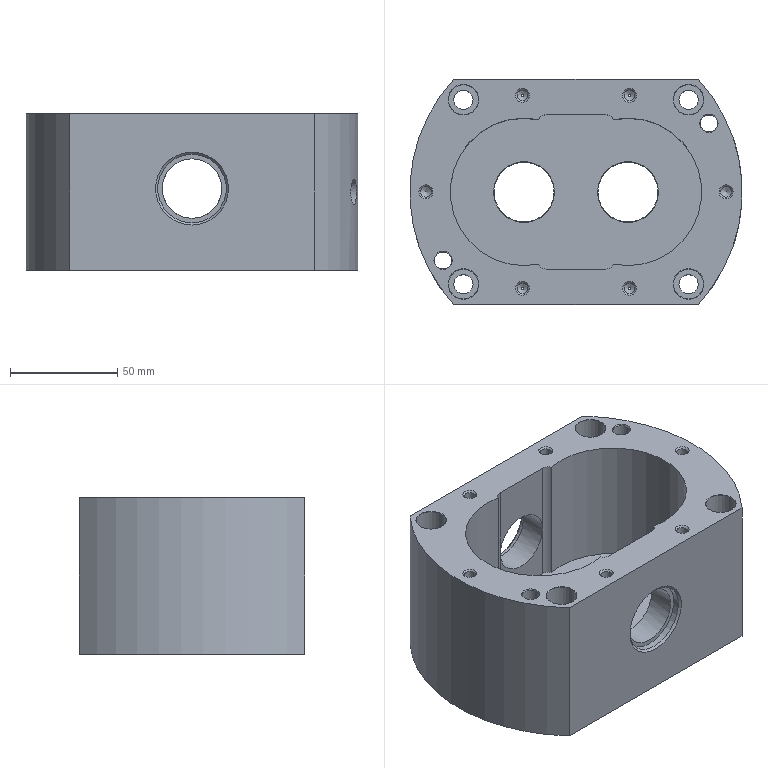NC program | NX | posted with a generic post | part box 155 x 105 x 73.2 mm
Lines 21970 to 22392 of 150882:
(FLOOR_WALL_2 , TOOL : D6JING)
N43890 T16 M6
N43892 G54
N43894 G17 G0 G90 X40.24 Y-44.486 B0. C0. S5000 M3
N43896 G43 Z30. H16
N43898 Z-1.
N43900 G94 G1 Z-2. F1000.
N43902 G3 X40.7 Y-44.7 R0.6
N43904 G1 X-40.7
N43906 Y-40.105
N43908 G3 X-40.188 Y-38.45 R6.3
N43910 G1 X-39.834 Y-36.282
N43912 G3 X-39.995 Y-35.966 R0.3
N43914 G1 X-41.955 Y-34.974
N43916 G2 X-49.587 Y-29.911 R39.2
N43918 G1 X-51.263 Y-28.491
N43920 G3 X-51.617 Y-28.466 R0.3
N43922 G1 X-53.477 Y-29.635
N43924 G3 X-54.757 Y-30.7 R6.3
N43926 G1 X-62.575
N43928 G2 X-66.236 Y21.7 R69.7
N43930 G1 X-61.75
N43932 G3 X-60.197 Y20.982 R6.3
N43934 G1 X-58.097 Y20.338
N43936 G3 X-57.762 Y20.455 R0.3
N43938 G1 X-56.515 Y22.263
N43940 G2 X-41.955 Y34.974 R39.2
N43942 G1 X-39.995 Y35.966
N43944 G3 X-39.834 Y36.282 R0.3
N43946 G1 X-40.188 Y38.45
N43948 G3 X-40.7 Y40.105 R6.3
N43950 G1 Y44.7
N43952 X40.7
N43954 Y40.105
N43956 G3 X40.188 Y38.45 R6.3
N43958 G1 X39.834 Y36.282
N43960 G3 X39.995 Y35.966 R0.3
N43962 G1 X41.955 Y34.974
N43964 G2 X49.587 Y29.911 R39.2
N43966 G1 X51.263 Y28.491
N43968 G3 X51.617 Y28.466 R0.3
N43970 G1 X53.477 Y29.635
N43972 G3 X54.757 Y30.7 R6.3
N43974 G1 X62.575
N43976 G2 X66.236 Y-21.7 R69.7
N43978 G1 X61.75
N43980 G3 X60.197 Y-20.982 R6.3
N43982 G1 X58.097 Y-20.338
N43984 G3 X57.762 Y-20.455 R0.3
N43986 G1 X56.515 Y-22.263
N43988 G2 X41.955 Y-34.974 R39.2
N43990 G1 X39.995 Y-35.966
N43992 G3 X39.834 Y-36.282 R0.3
N43994 G1 X40.188 Y-38.45
N43996 G3 X40.7 Y-40.105 R6.3
N43998 G1 Y-44.7
N44000 X37.7 Y-41.7
N44002 X-37.7
N44004 Y-40.705
N44006 G3 X-37.228 Y-38.934 R9.3
N44008 G1 X-36.874 Y-36.766
N44010 G3 X-38.64 Y-33.29 R3.3
N44012 G1 X-40.6 Y-32.297
N44014 G2 X-47.648 Y-27.622 R36.2
N44016 G1 X-49.324 Y-26.202
N44018 G3 X-53.214 Y-25.926 R3.3
N44020 G1 X-55.073 Y-27.095
N44022 G3 X-55.925 Y-27.7 R9.3
N44024 G1 X-60.676
N44026 G2 X-64.025 Y18.7 R66.7
N44028 G1 X-62.537
N44030 G3 X-61.076 Y18.113 R9.3
N44032 G1 X-58.976 Y17.47
N44034 G3 X-57.242 Y17.415 R3.3
N44036 G1 X-56.545 Y14.498
N44038 G3 X-51.643 Y-22.423 R35.4
N44040 X-54.876 Y-23.427 R6.3
N44042 G1 X-56.67 Y-24.555
N44044 G3 X-56.895 Y-24.7 R12.3
N44046 G1 X-58.716
N44048 G2 X-60.542 Y-19.808 R63.7
N44050 G1 X-57.691 Y-18.876
N44052 G3 X-56.472 Y-20.887 R38.4
N44054 G1 X-56.895 Y-21.153
N44056 G2 X-57.691 Y-18.876 R60.7
N44058 G1 X-60.542 Y-19.808
N44060 G2 X-61.856 Y15.215 R63.7
N44062 G1 X-59.854 Y14.601
N44064 G3 X-56.545 Y14.498 R6.3
N44066 G1 X-57.242 Y17.415
N44068 G3 X-55.293 Y18.751 R3.3
N44070 G1 X-54.045 Y20.559
N44072 G2 X-40.6 Y32.297 R36.2
N44074 G1 X-38.64 Y33.29
N44076 G3 X-36.874 Y36.766 R3.3
N44078 G1 X-37.228 Y38.934
N44080 G3 X-37.7 Y40.705 R9.3
N44082 G1 Y41.7
N44084 X37.7
N44086 Y40.705
N44088 G3 X37.228 Y38.934 R9.3
N44090 G1 X36.874 Y36.766
N44092 G3 X37.054 Y35.041 R3.3
N44094 G1 X34.257 Y33.956
N44096 G3 X1.238 Y26.9 R35.4
N44098 G1 X-1.238
N44100 G3 X-34.257 Y33.956 R35.4
N44102 X-33.913 Y37.249 R6.3
N44104 G1 X-34.15 Y38.7
N44106 X10.105
N44108 Y35.7
N44110 G3 X0.155 Y29.9 R38.4
N44112 G1 X-0.155
N44114 G3 X-10.105 Y35.7 R38.4
N44116 G1 X10.105
N44118 Y38.7
N44120 X34.15
N44122 X33.913 Y37.249
N44124 G3 X34.257 Y33.956 R6.3
N44126 G1 X37.054 Y35.041
N44128 G3 X38.64 Y33.29 R3.3
N44130 G1 X40.6 Y32.297
N44132 G2 X47.648 Y27.622 R36.2
N44134 G1 X49.324 Y26.202
N44136 G3 X53.214 Y25.926 R3.3
N44138 G1 X55.073 Y27.095
N44140 G3 X55.925 Y27.7 R9.3
N44142 G1 X60.676
N44144 G2 X64.025 Y-18.7 R66.7
N44146 G1 X62.537
N44148 G3 X61.076 Y-18.113 R9.3
N44150 G1 X58.976 Y-17.47
N44152 G3 X57.242 Y-17.415 R3.3
N44154 G1 X56.545 Y-14.498
N44156 G3 X51.643 Y22.423 R35.4
N44158 X54.876 Y23.427 R6.3
N44160 G1 X56.67 Y24.555
N44162 G3 X56.895 Y24.7 R12.3
N44164 G1 X58.716
N44166 G2 X60.542 Y19.809 R63.7
N44168 G1 X57.691 Y18.876
N44170 G3 X56.472 Y20.887 R38.4
N44172 G1 X56.895 Y21.153
N44174 G2 X57.691 Y18.876 R60.7
N44176 G1 X60.542 Y19.809
N44178 G2 X61.856 Y-15.215 R63.7
N44180 G1 X59.854 Y-14.601
N44182 G3 X56.545 Y-14.498 R6.3
N44184 G1 X57.242 Y-17.415
N44186 G3 X55.293 Y-18.751 R3.3
N44188 G1 X54.045 Y-20.559
N44190 G2 X40.6 Y-32.297 R36.2
N44192 G1 X38.64 Y-33.29
N44194 G3 X36.874 Y-36.766 R3.3
N44196 G1 X37.228 Y-38.934
N44198 G3 X37.7 Y-40.705 R9.3
N44200 G1 Y-41.7
N44202 X34.15 Y-38.7
N44204 X-34.15
N44206 X-33.913 Y-37.249
N44208 G3 X-34.257 Y-33.956 R6.3
N44210 X-1.238 Y-26.9 R35.4
N44212 G1 X1.238
N44214 G3 X11.21 Y-32.911 R35.4
N44216 G1 X10.105 Y-35.7
N44218 X-10.105
N44220 G3 X-0.155 Y-29.9 R38.4
N44222 G1 X0.155
N44224 G3 X10.105 Y-35.7 R38.4
N44226 G1 X11.21 Y-32.911
N44228 G3 X34.257 Y-33.956 R35.4
N44230 G1 X34.087 Y-33.381
N44232 G2 X1.461 Y-26.3 R34.8
N44234 G1 X-1.461
N44236 G2 X-1.461 Y26.3 R-34.8
N44238 G1 X1.461
N44240 G2 X34.087 Y-33.381 R-34.8
N44242 G1 X34.257 Y-33.956
N44244 G3 X33.913 Y-37.249 R6.3
N44246 G1 X34.15 Y-38.7
N44248 X33.298 Y-33.517
N44250 G3 X32.8 Y-33.424 R0.6
N44252 G2 X1.573 Y-26. R34.5
N44254 G1 X-1.573
N44256 G2 X-1.573 Y26. R-34.5
N44258 G1 X1.573
N44260 G2 X32.8 Y-33.424 R-34.5
N44262 G3 X32.408 Y-33.745 R0.6
N44264 G1 X31.809 Y-34.993
N44266 Z-1.
N44268 G0 Z30.
N44270 X-1.371 Y-43.7
N44272 Z-1.
N44274 G1 Z-2.
N44276 X-0.46 Y-44.786
N44278 G3 X0. Y-45. R0.6
N44280 G1 X41.
N44282 Y-40.037
N44284 G2 X40.485 Y-38.402 R6.
N44286 G1 X40.13 Y-36.234
N44288 X42.09 Y-35.242
N44290 G3 X56.762 Y-22.433 R39.5
N44292 G1 X58.009 Y-20.625
N44294 X60.109 Y-21.268
N44296 G2 X61.661 Y-22. R6.
N44298 G1 X66.453
N44300 G3 X62.761 Y31. R70.
N44302 G1 X54.624
N44304 G2 X53.317 Y29.889 R6.
N44306 G1 X51.457 Y28.72
N44308 X49.781 Y30.14
N44310 G3 X42.09 Y35.242 R39.5
N44312 G1 X40.13 Y36.234
N44314 X40.485 Y38.402
N44316 G2 X41. Y40.037 R6.
N44318 G1 Y45.
N44320 X-41.
N44322 Y40.037
N44324 G2 X-40.485 Y38.402 R6.
N44326 G1 X-40.13 Y36.234
N44328 X-42.09 Y35.242
N44330 G3 X-56.762 Y22.433 R39.5
N44332 G1 X-58.009 Y20.625
N44334 X-60.109 Y21.268
N44336 G2 X-61.661 Y22. R6.
N44338 G1 X-66.453
N44340 G3 X-62.761 Y-31. R70.
N44342 G1 X-54.624
N44344 G2 X-53.317 Y-29.889 R6.
N44346 G1 X-51.457 Y-28.72
N44348 X-49.781 Y-30.14
N44350 G3 X-42.09 Y-35.242 R39.5
N44352 G1 X-40.13 Y-36.234
N44354 X-40.485 Y-38.402
N44356 G2 X-41. Y-40.037 R6.
N44358 G1 Y-45.
N44360 X0.
N44362 G3 X0.46 Y-44.786 R0.6
N44364 G1 X1.119 Y-44.
N44366 Z-1.
N44368 G0 Z30.
N44370 X-60.222 Y-6.288
N44372 Z-6.
N44374 G1 Z-7.
N44376 G3 X-60.084 Y-5.8 R0.6
N44378 X-0.908 Y-27.8 R36.3
N44380 G1 X0.908
N44382 G3 X0.908 Y27.8 R-36.3
N44384 G1 X-0.908
N44386 G3 X-60.084 Y5.8 R36.3
N44388 G1 X-69.458
N44390 G2 X-66.236 Y21.7 R69.7
N44392 G1 X-61.75
N44394 G3 X-59.002 Y20.739 R6.3
N44396 G1 X-59.311 Y17.755
N44398 G3 X-62.552 Y8.8 R39.3
N44400 G1 X-66.117
N44402 G2 X-64.025 Y18.7 R66.7
N44404 G1 X-62.537
N44406 G3 X-59.311 Y17.755 R9.3
N44408 G1 X-59.002 Y20.739
N44410 G3 X-53.413 Y23.094 R6.3
N44412 G2 X-43.197 Y32.013 R37.2
N44414 G3 X-40.7 Y40.105 R6.3
N44416 G1 Y44.7
N44418 X-5.8
N44420 Y39.
N44422 G3 X-5.5 Y38.7 R0.3
N44424 G1 X5.5
N44426 G3 X5.8 Y39. R0.3
N44428 G1 Y44.7
N44430 X40.7
N44432 Y40.105
N44434 G3 X40.109 Y37.232 R6.3
N44436 G1 X37.111 Y37.136
N44438 G3 X0. Y30.926 R39.3
N44440 X-37.111 Y37.136 R39.3
N44442 X-37.7 Y40.705 R9.3
N44444 G1 Y41.7
N44446 X-8.8
N44448 Y39.
N44450 G3 X-5.5 Y35.7 R3.3
N44452 G1 X5.5
N44454 G3 X8.8 Y39. R3.3
N44456 G1 Y41.7
N44458 X37.7
N44460 Y40.705
N44462 G3 X37.111 Y37.136 R9.3
N44464 G1 X40.109 Y37.232
N44466 G3 X43.197 Y32.013 R6.3
N44468 G2 X46.376 Y29.904 R37.2
N44470 G3 X54.757 Y30.7 R6.3
N44472 G1 X62.575
N44474 G2 X69.458 Y5.8 R69.7
N44476 G1 X62.552
N44478 Y8.8
N44480 G3 X53.463 Y26.289 R39.3
N44482 X55.925 Y27.7 R9.3
N44484 G1 X60.676
N44486 G2 X61.67 Y25.411 R66.7
N44488 G1 X58.896 Y24.268
N44490 G3 X58.589 Y24.7 R42.3
N44492 G1 X58.716
N44494 G2 X58.896 Y24.268 R63.7
N44496 G1 X61.67 Y25.411
N44498 G2 X66.117 Y8.8 R66.7
N44500 G1 X62.552
N44502 Y5.8
N44504 X62.
N44506 G3 X61.7 Y5.5 R0.3
N44508 G1 Y-5.5
N44510 G3 X62. Y-5.8 R0.3
N44512 G1 X69.458
N44514 G2 X66.236 Y-21.7 R69.7
N44516 G1 X61.75
N44518 G3 X59.002 Y-20.739 R6.3
N44520 G1 X59.311 Y-17.755
N44522 G3 X62.552 Y-8.8 R39.3
N44524 G1 X66.117
N44526 G2 X64.025 Y-18.7 R66.7
N44528 G1 X62.537
N44530 G3 X59.311 Y-17.755 R9.3
N44532 G1 X59.002 Y-20.739
N44534 G3 X53.413 Y-23.094 R6.3
N44536 G2 X43.197 Y-32.013 R37.2
N44538 G3 X40.7 Y-40.105 R6.3
N44540 G1 Y-44.7
N44542 X5.8
N44544 Y-39.
N44546 G3 X5.5 Y-38.7 R0.3
N44548 G1 X-5.5
N44550 G3 X-5.8 Y-39. R0.3
N44552 G1 Y-44.7
N44554 X-40.7
N44556 Y-40.105
N44558 G3 X-40.109 Y-37.232 R6.3
N44560 G1 X-37.111 Y-37.136
N44562 G3 X0. Y-30.926 R39.3
N44564 X37.111 Y-37.136 R39.3
N44566 X37.7 Y-40.705 R9.3
N44568 G1 Y-41.7
N44570 X8.8
N44572 Y-39.
N44574 G3 X5.5 Y-35.7 R3.3
N44576 G1 X-5.5
N44578 G3 X-8.8 Y-39. R3.3
N44580 G1 Y-41.7
N44582 X-37.7
N44584 Y-40.705
N44586 G3 X-37.111 Y-37.136 R9.3
N44588 G1 X-40.109 Y-37.232
N44590 G3 X-43.197 Y-32.013 R6.3
N44592 G2 X-46.376 Y-29.904 R37.2
N44594 G3 X-54.757 Y-30.7 R6.3
N44596 G1 X-62.575
N44598 G2 X-69.458 Y-5.8 R69.7
N44600 G1 X-60.084
N44602 X-62.552 Y-8.8
N44604 G3 X-53.463 Y-26.289 R39.3
N44606 X-55.925 Y-27.7 R9.3
N44608 G1 X-60.676
N44610 G2 X-61.67 Y-25.411 R66.7
N44612 G1 X-58.896 Y-24.268
N44614 G3 X-58.589 Y-24.7 R42.3
N44616 G1 X-58.716
N44618 G2 X-58.896 Y-24.268 R63.7
N44620 G1 X-61.67 Y-25.411
N44622 G2 X-66.117 Y-8.8 R66.7
N44624 G1 X-62.552
N44626 X-59.442 Y-8.557
N44628 G3 X-59.336 Y-8.061 R0.6
N44630 G2 X-59.827 Y-5.5 R36.
N44632 G1 X-69.784
N44634 G3 X-62.761 Y-31. R70.
N44636 G1 X-54.624
N44638 G2 X-46.555 Y-30.145 R6.
N44640 G3 X-43.35 Y-32.271 R37.5
N44642 G2 X-41. Y-40.037 R6.
N44644 G1 Y-45.
N44646 X-5.5
N44648 Y-39.
N44650 X5.5
N44652 Y-45.
N44654 X41.
N44656 Y-40.037
N44658 G2 X43.35 Y-32.271 R6.
N44660 G3 X53.648 Y-23.281 R37.5
N44662 G2 X61.661 Y-22. R6.
N44664 G1 X66.453
N44666 G3 X69.784 Y-5.5 R70.
N44668 G1 X62.
N44670 Y5.5
N44672 X69.784
N44674 G3 X62.761 Y31. R70.
N44676 G1 X54.624
N44678 G2 X46.555 Y30.145 R6.
N44680 G3 X43.35 Y32.271 R37.5
N44682 G2 X41. Y40.037 R6.
N44684 G1 Y45.
N44686 X5.5
N44688 Y39.
N44690 X-5.5
N44692 Y45.
N44694 X-41.
N44696 Y40.037
N44698 G2 X-43.35 Y32.271 R6.
N44700 G3 X-53.648 Y23.281 R37.5
N44702 G2 X-61.661 Y22. R6.
N44704 G1 X-66.453
N44706 G3 X-69.784 Y5.5 R70.
N44708 G1 X-59.827
N44710 G2 X-1.017 Y27.5 R36.
N44712 G1 X1.017
N44714 G2 X1.017 Y-27.5 R-36.
N44716 G1 X-1.017
N44718 G2 X-59.336 Y-8.061 R36.
N44720 G3 X-59.648 Y-7.661 R0.6
N44722 G1 X-60.542 Y-7.204
N44724 Z-6.
N44726 G0 Z30.
N44728 M5